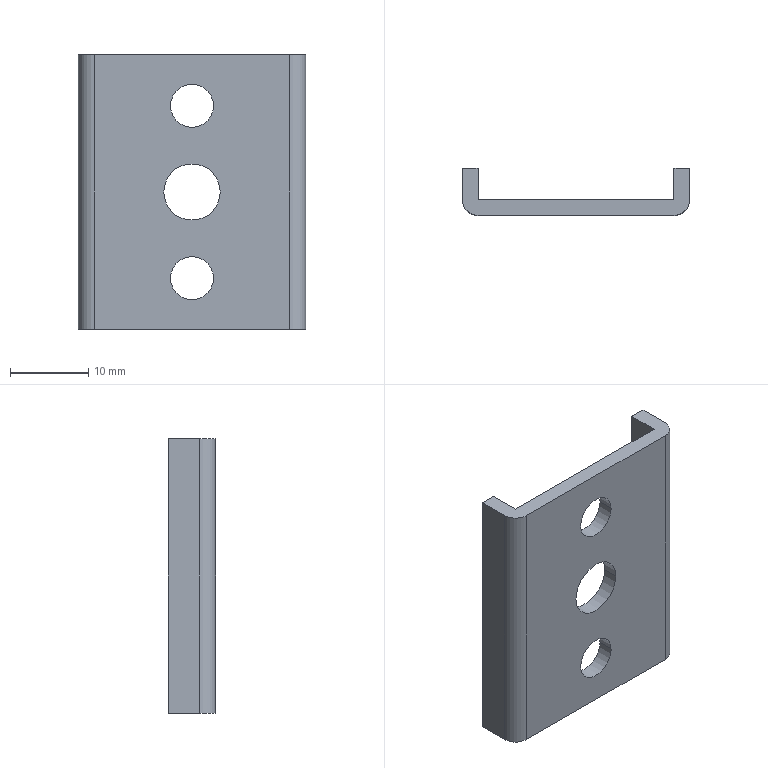Part | STEP file | _X2_751F4E45_X0_MS731-1_X2_8F_9 | 1 solid | 18 faces | box 29 x 6 x 35 mm | volume 2353 mm3 | plane 10 | cylinder 8 | commonest cylinder face diameters 5.5 x4 4 x2 7.2 x2
STEP:
#1=CARTESIAN_POINT('',(0.,0.,0.));
#2=DIRECTION('',(0.,0.,1.));
#3=DIRECTION('',(1.,0.,0.));
#4=AXIS2_PLACEMENT_3D('',#1,#2,#3);
#5=CARTESIAN_POINT('',(30.,20.681,-54.5));
#6=VERTEX_POINT('',#5);
#7=CARTESIAN_POINT('',(28.,20.681,-54.5));
#8=VERTEX_POINT('',#7);
#9=CARTESIAN_POINT('',(30.,20.681,-54.5));
#10=DIRECTION('',(-1.,0.,0.));
#11=VECTOR('',#10,1.);
#12=LINE('',#9,#11);
#13=CARTESIAN_POINT('',(15.5,20.681,-72.));
#14=DIRECTION('',(0.,-1.,0.));
#15=DIRECTION('',(1.,0.,0.));
#16=AXIS2_PLACEMENT_3D('',#13,#14,#15);
#17=PLANE('',#16);
#18=CARTESIAN_POINT('',(14.5,17.5));
#19=DIRECTION('',(-1.,0.));
#20=VECTOR('',#19,1.);
#21=LINE('',#18,#20);
#22=(GEOMETRIC_REPRESENTATION_CONTEXT(2)PARAMETRIC_REPRESENTATION_CONTEXT()REPRESENTATION_CONTEXT('',''));
#23=DEFINITIONAL_REPRESENTATION('',(#21),#22);
#24=PCURVE('',#17,#23);
#25=CARTESIAN_POINT('',(30.,20.681,-54.5));
#26=DIRECTION('',(0.,0.,1.));
#27=DIRECTION('',(1.,0.,0.));
#28=AXIS2_PLACEMENT_3D('',#25,#26,#27);
#29=PLANE('',#28);
#30=CARTESIAN_POINT('',(0.,0.));
#31=DIRECTION('',(-1.,0.));
#32=VECTOR('',#31,1.);
#33=LINE('',#30,#32);
#34=(GEOMETRIC_REPRESENTATION_CONTEXT(2)PARAMETRIC_REPRESENTATION_CONTEXT()REPRESENTATION_CONTEXT('',''));
#35=DEFINITIONAL_REPRESENTATION('',(#33),#34);
#36=PCURVE('',#29,#35);
#37=SURFACE_CURVE('',#12,(#24,#36),.PCURVE_S1.);
#38=EDGE_CURVE('',#6,#8,#37,.T.);
#39=ORIENTED_EDGE('',*,*,#38,.T.);
#40=CARTESIAN_POINT('',(28.,20.681,-89.5));
#41=VERTEX_POINT('',#40);
#42=CARTESIAN_POINT('',(28.,20.681,-54.5));
#43=DIRECTION('',(0.,0.,-1.));
#44=VECTOR('',#43,1.);
#45=LINE('',#42,#44);
#46=CARTESIAN_POINT('',(12.5,17.5));
#47=DIRECTION('',(0.,-1.));
#48=VECTOR('',#47,1.);
#49=LINE('',#46,#48);
#50=(GEOMETRIC_REPRESENTATION_CONTEXT(2)PARAMETRIC_REPRESENTATION_CONTEXT()REPRESENTATION_CONTEXT('',''));
#51=DEFINITIONAL_REPRESENTATION('',(#49),#50);
#52=PCURVE('',#17,#51);
#53=CARTESIAN_POINT('',(28.,16.681,-54.5));
#54=DIRECTION('',(1.,0.,0.));
#55=DIRECTION('',(0.,-1.,0.));
#56=AXIS2_PLACEMENT_3D('',#53,#54,#55);
#57=PLANE('',#56);
#58=CARTESIAN_POINT('',(-4.,0.));
#59=DIRECTION('',(0.,1.));
#60=VECTOR('',#59,1.);
#61=LINE('',#58,#60);
#62=(GEOMETRIC_REPRESENTATION_CONTEXT(2)PARAMETRIC_REPRESENTATION_CONTEXT()REPRESENTATION_CONTEXT('',''));
#63=DEFINITIONAL_REPRESENTATION('',(#61),#62);
#64=PCURVE('',#57,#63);
#65=SURFACE_CURVE('',#45,(#52,#64),.PCURVE_S1.);
#66=EDGE_CURVE('',#8,#41,#65,.T.);
#67=ORIENTED_EDGE('',*,*,#66,.T.);
#68=CARTESIAN_POINT('',(30.,20.681,-89.5));
#69=VERTEX_POINT('',#68);
#70=CARTESIAN_POINT('',(28.,20.681,-89.5));
#71=DIRECTION('',(1.,0.,0.));
#72=VECTOR('',#71,1.);
#73=LINE('',#70,#72);
#74=CARTESIAN_POINT('',(12.5,-17.5));
#75=DIRECTION('',(1.,0.));
#76=VECTOR('',#75,1.);
#77=LINE('',#74,#76);
#78=(GEOMETRIC_REPRESENTATION_CONTEXT(2)PARAMETRIC_REPRESENTATION_CONTEXT()REPRESENTATION_CONTEXT('',''));
#79=DEFINITIONAL_REPRESENTATION('',(#77),#78);
#80=PCURVE('',#17,#79);
#81=CARTESIAN_POINT('',(1.,20.681,-89.5));
#82=DIRECTION('',(0.,0.,-1.));
#83=DIRECTION('',(-1.,0.,0.));
#84=AXIS2_PLACEMENT_3D('',#81,#82,#83);
#85=PLANE('',#84);
#86=CARTESIAN_POINT('',(-27.,0.));
#87=DIRECTION('',(-1.,0.));
#88=VECTOR('',#87,1.);
#89=LINE('',#86,#88);
#90=(GEOMETRIC_REPRESENTATION_CONTEXT(2)PARAMETRIC_REPRESENTATION_CONTEXT()REPRESENTATION_CONTEXT('',''));
#91=DEFINITIONAL_REPRESENTATION('',(#89),#90);
#92=PCURVE('',#85,#91);
#93=SURFACE_CURVE('',#73,(#80,#92),.PCURVE_S1.);
#94=EDGE_CURVE('',#41,#69,#93,.T.);
#95=ORIENTED_EDGE('',*,*,#94,.T.);
#96=CARTESIAN_POINT('',(30.,20.681,-89.5));
#97=DIRECTION('',(0.,0.,1.));
#98=VECTOR('',#97,1.);
#99=LINE('',#96,#98);
#100=CARTESIAN_POINT('',(14.5,-17.5));
#101=DIRECTION('',(0.,1.));
#102=VECTOR('',#101,1.);
#103=LINE('',#100,#102);
#104=(GEOMETRIC_REPRESENTATION_CONTEXT(2)PARAMETRIC_REPRESENTATION_CONTEXT()REPRESENTATION_CONTEXT('',''));
#105=DEFINITIONAL_REPRESENTATION('',(#103),#104);
#106=PCURVE('',#17,#105);
#107=CARTESIAN_POINT('',(30.,20.681,-89.5));
#108=DIRECTION('',(1.,0.,0.));
#109=DIRECTION('',(0.,0.,-1.));
#110=AXIS2_PLACEMENT_3D('',#107,#108,#109);
#111=PLANE('',#110);
#112=CARTESIAN_POINT('',(0.,0.));
#113=DIRECTION('',(-1.,0.));
#114=VECTOR('',#113,1.);
#115=LINE('',#112,#114);
#116=(GEOMETRIC_REPRESENTATION_CONTEXT(2)PARAMETRIC_REPRESENTATION_CONTEXT()REPRESENTATION_CONTEXT('',''));
#117=DEFINITIONAL_REPRESENTATION('',(#115),#116);
#118=PCURVE('',#111,#117);
#119=SURFACE_CURVE('',#99,(#106,#118),.PCURVE_S1.);
#120=EDGE_CURVE('',#69,#6,#119,.T.);
#121=ORIENTED_EDGE('',*,*,#120,.T.);
#122=EDGE_LOOP('',(#39,#67,#95,#121));
#123=FACE_BOUND('',#122,.F.);
#124=ADVANCED_FACE('',(#123),#17,.F.);
#125=CARTESIAN_POINT('',(28.,14.681,-54.5));
#126=VERTEX_POINT('',#125);
#127=CARTESIAN_POINT('',(3.,14.681,-54.5));
#128=VERTEX_POINT('',#127);
#129=CARTESIAN_POINT('',(28.,14.681,-54.5));
#130=DIRECTION('',(-1.,0.,0.));
#131=VECTOR('',#130,1.);
#132=LINE('',#129,#131);
#133=CARTESIAN_POINT('',(-2.,-6.));
#134=DIRECTION('',(-1.,0.));
#135=VECTOR('',#134,1.);
#136=LINE('',#133,#135);
#137=(GEOMETRIC_REPRESENTATION_CONTEXT(2)PARAMETRIC_REPRESENTATION_CONTEXT()REPRESENTATION_CONTEXT('',''));
#138=DEFINITIONAL_REPRESENTATION('',(#136),#137);
#139=PCURVE('',#29,#138);
#140=CARTESIAN_POINT('',(15.5,14.681,-72.));
#141=DIRECTION('',(0.,-1.,0.));
#142=DIRECTION('',(1.,0.,0.));
#143=AXIS2_PLACEMENT_3D('',#140,#141,#142);
#144=PLANE('',#143);
#145=CARTESIAN_POINT('',(12.5,17.5));
#146=DIRECTION('',(-1.,0.));
#147=VECTOR('',#146,1.);
#148=LINE('',#145,#147);
#149=(GEOMETRIC_REPRESENTATION_CONTEXT(2)PARAMETRIC_REPRESENTATION_CONTEXT()REPRESENTATION_CONTEXT('',''));
#150=DEFINITIONAL_REPRESENTATION('',(#148),#149);
#151=PCURVE('',#144,#150);
#152=SURFACE_CURVE('',#132,(#139,#151),.PCURVE_S1.);
#153=EDGE_CURVE('',#126,#128,#152,.T.);
#154=ORIENTED_EDGE('',*,*,#153,.T.);
#155=CARTESIAN_POINT('',(1.,16.681,-54.5));
#156=VERTEX_POINT('',#155);
#157=CARTESIAN_POINT('',(3.,16.681,-54.5));
#158=DIRECTION('',(0.,0.,1.));
#159=DIRECTION('',(-1.,0.,0.));
#160=AXIS2_PLACEMENT_3D('',#157,#158,#159);
#161=CIRCLE('',#160,2.);
#162=CARTESIAN_POINT('',(-27.,-4.));
#163=DIRECTION('',(-1.,0.));
#164=AXIS2_PLACEMENT_2D('',#162,#163);
#165=CIRCLE('',#164,2.);
#166=(GEOMETRIC_REPRESENTATION_CONTEXT(2)PARAMETRIC_REPRESENTATION_CONTEXT()REPRESENTATION_CONTEXT('',''));
#167=DEFINITIONAL_REPRESENTATION('',(#165),#166);
#168=PCURVE('',#29,#167);
#169=CARTESIAN_POINT('',(3.,16.681,-54.425));
#170=DIRECTION('',(0.,0.,-1.));
#171=DIRECTION('',(0.,1.,0.));
#172=AXIS2_PLACEMENT_3D('',#169,#170,#171);
#173=CYLINDRICAL_SURFACE('',#172,2.);
#174=CARTESIAN_POINT('',(4.712,0.0754));
#175=DIRECTION('',(-1.,0.));
#176=VECTOR('',#175,1.);
#177=LINE('',#174,#176);
#178=(GEOMETRIC_REPRESENTATION_CONTEXT(2)PARAMETRIC_REPRESENTATION_CONTEXT()REPRESENTATION_CONTEXT('',''));
#179=DEFINITIONAL_REPRESENTATION('',(#177),#178);
#180=PCURVE('',#173,#179);
#181=SURFACE_CURVE('',#161,(#168,#180),.PCURVE_S1.);
#182=EDGE_CURVE('',#156,#128,#181,.T.);
#183=ORIENTED_EDGE('',*,*,#182,.F.);
#184=CARTESIAN_POINT('',(1.,20.681,-54.5));
#185=VERTEX_POINT('',#184);
#186=CARTESIAN_POINT('',(1.,20.681,-54.5));
#187=DIRECTION('',(0.,-1.,0.));
#188=VECTOR('',#187,1.);
#189=LINE('',#186,#188);
#190=CARTESIAN_POINT('',(-29.,0.));
#191=DIRECTION('',(0.,-1.));
#192=VECTOR('',#191,1.);
#193=LINE('',#190,#192);
#194=(GEOMETRIC_REPRESENTATION_CONTEXT(2)PARAMETRIC_REPRESENTATION_CONTEXT()REPRESENTATION_CONTEXT('',''));
#195=DEFINITIONAL_REPRESENTATION('',(#193),#194);
#196=PCURVE('',#29,#195);
#197=CARTESIAN_POINT('',(1.,20.681,-54.5));
#198=DIRECTION('',(-1.,0.,0.));
#199=DIRECTION('',(0.,0.,1.));
#200=AXIS2_PLACEMENT_3D('',#197,#198,#199);
#201=PLANE('',#200);
#202=CARTESIAN_POINT('',(0.,0.));
#203=DIRECTION('',(0.,-1.));
#204=VECTOR('',#203,1.);
#205=LINE('',#202,#204);
#206=(GEOMETRIC_REPRESENTATION_CONTEXT(2)PARAMETRIC_REPRESENTATION_CONTEXT()REPRESENTATION_CONTEXT('',''));
#207=DEFINITIONAL_REPRESENTATION('',(#205),#206);
#208=PCURVE('',#201,#207);
#209=SURFACE_CURVE('',#189,(#196,#208),.PCURVE_S1.);
#210=EDGE_CURVE('',#185,#156,#209,.T.);
#211=ORIENTED_EDGE('',*,*,#210,.F.);
#212=CARTESIAN_POINT('',(3.,20.681,-54.5));
#213=VERTEX_POINT('',#212);
#214=CARTESIAN_POINT('',(3.,20.681,-54.5));
#215=DIRECTION('',(-1.,0.,0.));
#216=VECTOR('',#215,1.);
#217=LINE('',#214,#216);
#218=CARTESIAN_POINT('',(-27.,0.));
#219=DIRECTION('',(-1.,0.));
#220=VECTOR('',#219,1.);
#221=LINE('',#218,#220);
#222=(GEOMETRIC_REPRESENTATION_CONTEXT(2)PARAMETRIC_REPRESENTATION_CONTEXT()REPRESENTATION_CONTEXT('',''));
#223=DEFINITIONAL_REPRESENTATION('',(#221),#222);
#224=PCURVE('',#29,#223);
#225=CARTESIAN_POINT('',(15.5,20.681,-72.));
#226=DIRECTION('',(0.,-1.,0.));
#227=DIRECTION('',(1.,0.,0.));
#228=AXIS2_PLACEMENT_3D('',#225,#226,#227);
#229=PLANE('',#228);
#230=CARTESIAN_POINT('',(-12.5,17.5));
#231=DIRECTION('',(-1.,0.));
#232=VECTOR('',#231,1.);
#233=LINE('',#230,#232);
#234=(GEOMETRIC_REPRESENTATION_CONTEXT(2)PARAMETRIC_REPRESENTATION_CONTEXT()REPRESENTATION_CONTEXT('',''));
#235=DEFINITIONAL_REPRESENTATION('',(#233),#234);
#236=PCURVE('',#229,#235);
#237=SURFACE_CURVE('',#217,(#224,#236),.PCURVE_S1.);
#238=EDGE_CURVE('',#213,#185,#237,.T.);
#239=ORIENTED_EDGE('',*,*,#238,.F.);
#240=CARTESIAN_POINT('',(3.,16.681,-54.5));
#241=VERTEX_POINT('',#240);
#242=CARTESIAN_POINT('',(3.,20.681,-54.5));
#243=DIRECTION('',(0.,-1.,0.));
#244=VECTOR('',#243,1.);
#245=LINE('',#242,#244);
#246=CARTESIAN_POINT('',(-27.,0.));
#247=DIRECTION('',(0.,-1.));
#248=VECTOR('',#247,1.);
#249=LINE('',#246,#248);
#250=(GEOMETRIC_REPRESENTATION_CONTEXT(2)PARAMETRIC_REPRESENTATION_CONTEXT()REPRESENTATION_CONTEXT('',''));
#251=DEFINITIONAL_REPRESENTATION('',(#249),#250);
#252=PCURVE('',#29,#251);
#253=CARTESIAN_POINT('',(3.,20.681,-54.5));
#254=DIRECTION('',(-1.,0.,0.));
#255=DIRECTION('',(0.,1.,0.));
#256=AXIS2_PLACEMENT_3D('',#253,#254,#255);
#257=PLANE('',#256);
#258=CARTESIAN_POINT('',(0.,0.));
#259=DIRECTION('',(-1.,0.));
#260=VECTOR('',#259,1.);
#261=LINE('',#258,#260);
#262=(GEOMETRIC_REPRESENTATION_CONTEXT(2)PARAMETRIC_REPRESENTATION_CONTEXT()REPRESENTATION_CONTEXT('',''));
#263=DEFINITIONAL_REPRESENTATION('',(#261),#262);
#264=PCURVE('',#257,#263);
#265=SURFACE_CURVE('',#245,(#252,#264),.PCURVE_S1.);
#266=EDGE_CURVE('',#213,#241,#265,.T.);
#267=ORIENTED_EDGE('',*,*,#266,.T.);
#268=CARTESIAN_POINT('',(28.,16.681,-54.5));
#269=VERTEX_POINT('',#268);
#270=CARTESIAN_POINT('',(3.,16.681,-54.5));
#271=DIRECTION('',(1.,0.,0.));
#272=VECTOR('',#271,1.);
#273=LINE('',#270,#272);
#274=CARTESIAN_POINT('',(-27.,-4.));
#275=DIRECTION('',(1.,0.));
#276=VECTOR('',#275,1.);
#277=LINE('',#274,#276);
#278=(GEOMETRIC_REPRESENTATION_CONTEXT(2)PARAMETRIC_REPRESENTATION_CONTEXT()REPRESENTATION_CONTEXT('',''));
#279=DEFINITIONAL_REPRESENTATION('',(#277),#278);
#280=PCURVE('',#29,#279);
#281=CARTESIAN_POINT('',(3.,16.681,-54.5));
#282=DIRECTION('',(0.,-1.,0.));
#283=DIRECTION('',(-1.,0.,0.));
#284=AXIS2_PLACEMENT_3D('',#281,#282,#283);
#285=PLANE('',#284);
#286=CARTESIAN_POINT('',(0.,0.));
#287=DIRECTION('',(-1.,0.));
#288=VECTOR('',#287,1.);
#289=LINE('',#286,#288);
#290=(GEOMETRIC_REPRESENTATION_CONTEXT(2)PARAMETRIC_REPRESENTATION_CONTEXT()REPRESENTATION_CONTEXT('',''));
#291=DEFINITIONAL_REPRESENTATION('',(#289),#290);
#292=PCURVE('',#285,#291);
#293=SURFACE_CURVE('',#273,(#280,#292),.PCURVE_S1.);
#294=EDGE_CURVE('',#241,#269,#293,.T.);
#295=ORIENTED_EDGE('',*,*,#294,.T.);
#296=CARTESIAN_POINT('',(28.,20.681,-54.5));
#297=DIRECTION('',(0.,-1.,0.));
#298=VECTOR('',#297,1.);
#299=LINE('',#296,#298);
#300=CARTESIAN_POINT('',(-2.,0.));
#301=DIRECTION('',(0.,-1.));
#302=VECTOR('',#301,1.);
#303=LINE('',#300,#302);
#304=(GEOMETRIC_REPRESENTATION_CONTEXT(2)PARAMETRIC_REPRESENTATION_CONTEXT()REPRESENTATION_CONTEXT('',''));
#305=DEFINITIONAL_REPRESENTATION('',(#303),#304);
#306=PCURVE('',#29,#305);
#307=CARTESIAN_POINT('',(-4.,0.));
#308=DIRECTION('',(1.,0.));
#309=VECTOR('',#308,1.);
#310=LINE('',#307,#309);
#311=(GEOMETRIC_REPRESENTATION_CONTEXT(2)PARAMETRIC_REPRESENTATION_CONTEXT()REPRESENTATION_CONTEXT('',''));
#312=DEFINITIONAL_REPRESENTATION('',(#310),#311);
#313=PCURVE('',#57,#312);
#314=SURFACE_CURVE('',#299,(#306,#313),.PCURVE_S1.);
#315=EDGE_CURVE('',#8,#269,#314,.T.);
#316=ORIENTED_EDGE('',*,*,#315,.F.);
#317=ORIENTED_EDGE('',*,*,#38,.F.);
#318=CARTESIAN_POINT('',(30.,16.681,-54.5));
#319=VERTEX_POINT('',#318);
#320=CARTESIAN_POINT('',(30.,20.681,-54.5));
#321=DIRECTION('',(0.,-1.,0.));
#322=VECTOR('',#321,1.);
#323=LINE('',#320,#322);
#324=CARTESIAN_POINT('',(0.,0.));
#325=DIRECTION('',(0.,-1.));
#326=VECTOR('',#325,1.);
#327=LINE('',#324,#326);
#328=(GEOMETRIC_REPRESENTATION_CONTEXT(2)PARAMETRIC_REPRESENTATION_CONTEXT()REPRESENTATION_CONTEXT('',''));
#329=DEFINITIONAL_REPRESENTATION('',(#327),#328);
#330=PCURVE('',#29,#329);
#331=CARTESIAN_POINT('',(-35.,0.));
#332=DIRECTION('',(0.,-1.));
#333=VECTOR('',#332,1.);
#334=LINE('',#331,#333);
#335=(GEOMETRIC_REPRESENTATION_CONTEXT(2)PARAMETRIC_REPRESENTATION_CONTEXT()REPRESENTATION_CONTEXT('',''));
#336=DEFINITIONAL_REPRESENTATION('',(#334),#335);
#337=PCURVE('',#111,#336);
#338=SURFACE_CURVE('',#323,(#330,#337),.PCURVE_S1.);
#339=EDGE_CURVE('',#6,#319,#338,.T.);
#340=ORIENTED_EDGE('',*,*,#339,.T.);
#341=CARTESIAN_POINT('',(28.,16.681,-54.5));
#342=DIRECTION('',(0.,0.,1.));
#343=DIRECTION('',(0.,-1.,0.));
#344=AXIS2_PLACEMENT_3D('',#341,#342,#343);
#345=CIRCLE('',#344,2.);
#346=CARTESIAN_POINT('',(-2.,-4.));
#347=DIRECTION('',(0.,-1.));
#348=AXIS2_PLACEMENT_2D('',#346,#347);
#349=CIRCLE('',#348,2.);
#350=(GEOMETRIC_REPRESENTATION_CONTEXT(2)PARAMETRIC_REPRESENTATION_CONTEXT()REPRESENTATION_CONTEXT('',''));
#351=DEFINITIONAL_REPRESENTATION('',(#349),#350);
#352=PCURVE('',#29,#351);
#353=CARTESIAN_POINT('',(28.,16.681,-89.577));
#354=DIRECTION('',(0.,0.,1.));
#355=DIRECTION('',(0.,1.,0.));
#356=AXIS2_PLACEMENT_3D('',#353,#354,#355);
#357=CYLINDRICAL_SURFACE('',#356,2.);
#358=CARTESIAN_POINT('',(3.142,35.077));
#359=DIRECTION('',(1.,0.));
#360=VECTOR('',#359,1.);
#361=LINE('',#358,#360);
#362=(GEOMETRIC_REPRESENTATION_CONTEXT(2)PARAMETRIC_REPRESENTATION_CONTEXT()REPRESENTATION_CONTEXT('',''));
#363=DEFINITIONAL_REPRESENTATION('',(#361),#362);
#364=PCURVE('',#357,#363);
#365=SURFACE_CURVE('',#345,(#352,#364),.PCURVE_S1.);
#366=EDGE_CURVE('',#126,#319,#365,.T.);
#367=ORIENTED_EDGE('',*,*,#366,.F.);
#368=EDGE_LOOP('',(#154,#183,#211,#239,#267,#295,#316,#317,#340,#367));
#369=FACE_BOUND('',#368,.F.);
#370=ADVANCED_FACE('',(#369),#29,.T.);
#371=CARTESIAN_POINT('',(3.,14.681,-89.5));
#372=VERTEX_POINT('',#371);
#373=CARTESIAN_POINT('',(28.,14.681,-89.5));
#374=VERTEX_POINT('',#373);
#375=CARTESIAN_POINT('',(3.,14.681,-89.5));
#376=DIRECTION('',(1.,0.,0.));
#377=VECTOR('',#376,1.);
#378=LINE('',#375,#377);
#379=CARTESIAN_POINT('',(-12.5,-17.5));
#380=DIRECTION('',(1.,0.));
#381=VECTOR('',#380,1.);
#382=LINE('',#379,#381);
#383=(GEOMETRIC_REPRESENTATION_CONTEXT(2)PARAMETRIC_REPRESENTATION_CONTEXT()REPRESENTATION_CONTEXT('',''));
#384=DEFINITIONAL_REPRESENTATION('',(#382),#383);
#385=PCURVE('',#144,#384);
#386=CARTESIAN_POINT('',(-2.,-6.));
#387=DIRECTION('',(-1.,0.));
#388=VECTOR('',#387,1.);
#389=LINE('',#386,#388);
#390=(GEOMETRIC_REPRESENTATION_CONTEXT(2)PARAMETRIC_REPRESENTATION_CONTEXT()REPRESENTATION_CONTEXT('',''));
#391=DEFINITIONAL_REPRESENTATION('',(#389),#390);
#392=PCURVE('',#85,#391);
#393=SURFACE_CURVE('',#378,(#385,#392),.PCURVE_S1.);
#394=EDGE_CURVE('',#372,#374,#393,.T.);
#395=ORIENTED_EDGE('',*,*,#394,.F.);
#396=CARTESIAN_POINT('',(3.,14.681,-89.5));
#397=DIRECTION('',(0.,0.,1.));
#398=VECTOR('',#397,1.);
#399=LINE('',#396,#398);
#400=CARTESIAN_POINT('',(-12.5,-17.5));
#401=DIRECTION('',(0.,1.));
#402=VECTOR('',#401,1.);
#403=LINE('',#400,#402);
#404=(GEOMETRIC_REPRESENTATION_CONTEXT(2)PARAMETRIC_REPRESENTATION_CONTEXT()REPRESENTATION_CONTEXT('',''));
#405=DEFINITIONAL_REPRESENTATION('',(#403),#404);
#406=PCURVE('',#144,#405);
#407=CARTESIAN_POINT('',(3.142,35.075));
#408=DIRECTION('',(0.,-1.));
#409=VECTOR('',#408,1.);
#410=LINE('',#407,#409);
#411=(GEOMETRIC_REPRESENTATION_CONTEXT(2)PARAMETRIC_REPRESENTATION_CONTEXT()REPRESENTATION_CONTEXT('',''));
#412=DEFINITIONAL_REPRESENTATION('',(#410),#411);
#413=PCURVE('',#173,#412);
#414=SURFACE_CURVE('',#399,(#406,#413),.PCURVE_S1.);
#415=EDGE_CURVE('',#372,#128,#414,.T.);
#416=ORIENTED_EDGE('',*,*,#415,.T.);
#417=ORIENTED_EDGE('',*,*,#153,.F.);
#418=CARTESIAN_POINT('',(28.,14.681,-54.5));
#419=DIRECTION('',(0.,0.,-1.));
#420=VECTOR('',#419,1.);
#421=LINE('',#418,#420);
#422=CARTESIAN_POINT('',(12.5,17.5));
#423=DIRECTION('',(0.,-1.));
#424=VECTOR('',#423,1.);
#425=LINE('',#422,#424);
#426=(GEOMETRIC_REPRESENTATION_CONTEXT(2)PARAMETRIC_REPRESENTATION_CONTEXT()REPRESENTATION_CONTEXT('',''));
#427=DEFINITIONAL_REPRESENTATION('',(#425),#426);
#428=PCURVE('',#144,#427);
#429=CARTESIAN_POINT('',(3.142,35.077));
#430=DIRECTION('',(0.,-1.));
#431=VECTOR('',#430,1.);
#432=LINE('',#429,#431);
#433=(GEOMETRIC_REPRESENTATION_CONTEXT(2)PARAMETRIC_REPRESENTATION_CONTEXT()REPRESENTATION_CONTEXT('',''));
#434=DEFINITIONAL_REPRESENTATION('',(#432),#433);
#435=PCURVE('',#357,#434);
#436=SURFACE_CURVE('',#421,(#428,#435),.PCURVE_S1.);
#437=EDGE_CURVE('',#126,#374,#436,.T.);
#438=ORIENTED_EDGE('',*,*,#437,.T.);
#439=EDGE_LOOP('',(#395,#416,#417,#438));
#440=FACE_BOUND('',#439,.F.);
#441=CARTESIAN_POINT('',(18.25,14.681,-83.));
#442=VERTEX_POINT('',#441);
#443=CARTESIAN_POINT('',(12.75,14.681,-83.));
#444=VERTEX_POINT('',#443);
#445=CARTESIAN_POINT('',(15.5,14.681,-83.));
#446=DIRECTION('',(0.,1.,0.));
#447=DIRECTION('',(1.,0.,0.));
#448=AXIS2_PLACEMENT_3D('',#445,#446,#447);
#449=CIRCLE('',#448,2.75);
#450=CARTESIAN_POINT('',(2.75,-11.));
#451=CARTESIAN_POINT('',(2.75,-15.763));
#452=CARTESIAN_POINT('',(-1.375,-13.382));
#453=CARTESIAN_POINT('',(-5.5,-11.));
#454=CARTESIAN_POINT('',(-1.375,-8.618));
#455=CARTESIAN_POINT('',(2.75,-6.237));
#456=CARTESIAN_POINT('',(2.75,-11.));
#457=(BOUNDED_CURVE()B_SPLINE_CURVE(2,(#450,#451,#452,#453,#454,#455,#456),.UNSPECIFIED.,.T.,.F.)B_SPLINE_CURVE_WITH_KNOTS((1,2,2,2,2,1),(-2.094,0.,2.094,4.189,6.283,8.378),.UNSPECIFIED.)CURVE()GEOMETRIC_REPRESENTATION_ITEM()RATIONAL_B_SPLINE_CURVE((1.,0.5,1.,0.5,1.,0.5,1.))REPRESENTATION_ITEM(''));
#458=(GEOMETRIC_REPRESENTATION_CONTEXT(2)PARAMETRIC_REPRESENTATION_CONTEXT()REPRESENTATION_CONTEXT('',''));
#459=DEFINITIONAL_REPRESENTATION('',(#457),#458);
#460=PCURVE('',#144,#459);
#461=CARTESIAN_POINT('',(15.5,20.681,-83.));
#462=DIRECTION('',(0.,-1.,0.));
#463=DIRECTION('',(1.,0.,0.));
#464=AXIS2_PLACEMENT_3D('',#461,#462,#463);
#465=CYLINDRICAL_SURFACE('',#464,2.75);
#466=CARTESIAN_POINT('',(6.283,6.));
#467=DIRECTION('',(-1.,0.));
#468=VECTOR('',#467,1.);
#469=LINE('',#466,#468);
#470=(GEOMETRIC_REPRESENTATION_CONTEXT(2)PARAMETRIC_REPRESENTATION_CONTEXT()REPRESENTATION_CONTEXT('',''));
#471=DEFINITIONAL_REPRESENTATION('',(#469),#470);
#472=PCURVE('',#465,#471);
#473=SURFACE_CURVE('',#449,(#460,#472),.PCURVE_S1.);
#474=EDGE_CURVE('',#442,#444,#473,.T.);
#475=ORIENTED_EDGE('',*,*,#474,.F.);
#476=CARTESIAN_POINT('',(15.5,14.681,-83.));
#477=DIRECTION('',(0.,1.,0.));
#478=DIRECTION('',(-1.,0.,0.));
#479=AXIS2_PLACEMENT_3D('',#476,#477,#478);
#480=CIRCLE('',#479,2.75);
#481=CARTESIAN_POINT('',(-2.75,-11.));
#482=CARTESIAN_POINT('',(-2.75,-6.237));
#483=CARTESIAN_POINT('',(1.375,-8.618));
#484=CARTESIAN_POINT('',(5.5,-11.));
#485=CARTESIAN_POINT('',(1.375,-13.382));
#486=CARTESIAN_POINT('',(-2.75,-15.763));
#487=CARTESIAN_POINT('',(-2.75,-11.));
#488=(BOUNDED_CURVE()B_SPLINE_CURVE(2,(#481,#482,#483,#484,#485,#486,#487),.UNSPECIFIED.,.T.,.F.)B_SPLINE_CURVE_WITH_KNOTS((1,2,2,2,2,1),(-2.094,0.,2.094,4.189,6.283,8.378),.UNSPECIFIED.)CURVE()GEOMETRIC_REPRESENTATION_ITEM()RATIONAL_B_SPLINE_CURVE((1.,0.5,1.,0.5,1.,0.5,1.))REPRESENTATION_ITEM(''));
#489=(GEOMETRIC_REPRESENTATION_CONTEXT(2)PARAMETRIC_REPRESENTATION_CONTEXT()REPRESENTATION_CONTEXT('',''));
#490=DEFINITIONAL_REPRESENTATION('',(#488),#489);
#491=PCURVE('',#144,#490);
#492=CARTESIAN_POINT('',(15.5,20.681,-83.));
#493=DIRECTION('',(0.,-1.,0.));
#494=DIRECTION('',(1.,0.,0.));
#495=AXIS2_PLACEMENT_3D('',#492,#493,#494);
#496=CYLINDRICAL_SURFACE('',#495,2.75);
#497=CARTESIAN_POINT('',(3.142,6.));
#498=DIRECTION('',(-1.,0.));
#499=VECTOR('',#498,1.);
#500=LINE('',#497,#499);
#501=(GEOMETRIC_REPRESENTATION_CONTEXT(2)PARAMETRIC_REPRESENTATION_CONTEXT()REPRESENTATION_CONTEXT('',''));
#502=DEFINITIONAL_REPRESENTATION('',(#500),#501);
#503=PCURVE('',#496,#502);
#504=SURFACE_CURVE('',#480,(#491,#503),.PCURVE_S1.);
#505=EDGE_CURVE('',#444,#442,#504,.T.);
#506=ORIENTED_EDGE('',*,*,#505,.F.);
#507=EDGE_LOOP('',(#475,#506));
#508=FACE_BOUND('',#507,.F.);
#509=CARTESIAN_POINT('',(18.25,14.681,-61.));
#510=VERTEX_POINT('',#509);
#511=CARTESIAN_POINT('',(12.75,14.681,-61.));
#512=VERTEX_POINT('',#511);
#513=CARTESIAN_POINT('',(15.5,14.681,-61.));
#514=DIRECTION('',(0.,1.,0.));
#515=DIRECTION('',(1.,0.,0.));
#516=AXIS2_PLACEMENT_3D('',#513,#514,#515);
#517=CIRCLE('',#516,2.75);
#518=CARTESIAN_POINT('',(2.75,11.));
#519=CARTESIAN_POINT('',(2.75,6.237));
#520=CARTESIAN_POINT('',(-1.375,8.618));
#521=CARTESIAN_POINT('',(-5.5,11.));
#522=CARTESIAN_POINT('',(-1.375,13.382));
#523=CARTESIAN_POINT('',(2.75,15.763));
#524=CARTESIAN_POINT('',(2.75,11.));
#525=(BOUNDED_CURVE()B_SPLINE_CURVE(2,(#518,#519,#520,#521,#522,#523,#524),.UNSPECIFIED.,.T.,.F.)B_SPLINE_CURVE_WITH_KNOTS((1,2,2,2,2,1),(-2.094,0.,2.094,4.189,6.283,8.378),.UNSPECIFIED.)CURVE()GEOMETRIC_REPRESENTATION_ITEM()RATIONAL_B_SPLINE_CURVE((1.,0.5,1.,0.5,1.,0.5,1.))REPRESENTATION_ITEM(''));
#526=(GEOMETRIC_REPRESENTATION_CONTEXT(2)PARAMETRIC_REPRESENTATION_CONTEXT()REPRESENTATION_CONTEXT('',''));
#527=DEFINITIONAL_REPRESENTATION('',(#525),#526);
#528=PCURVE('',#144,#527);
#529=CARTESIAN_POINT('',(15.5,20.681,-61.));
#530=DIRECTION('',(0.,-1.,0.));
#531=DIRECTION('',(1.,0.,0.));
#532=AXIS2_PLACEMENT_3D('',#529,#530,#531);
#533=CYLINDRICAL_SURFACE('',#532,2.75);
#534=CARTESIAN_POINT('',(6.283,6.));
#535=DIRECTION('',(-1.,0.));
#536=VECTOR('',#535,1.);
#537=LINE('',#534,#536);
#538=(GEOMETRIC_REPRESENTATION_CONTEXT(2)PARAMETRIC_REPRESENTATION_CONTEXT()REPRESENTATION_CONTEXT('',''));
#539=DEFINITIONAL_REPRESENTATION('',(#537),#538);
#540=PCURVE('',#533,#539);
#541=SURFACE_CURVE('',#517,(#528,#540),.PCURVE_S1.);
#542=EDGE_CURVE('',#510,#512,#541,.T.);
#543=ORIENTED_EDGE('',*,*,#542,.F.);
#544=CARTESIAN_POINT('',(15.5,14.681,-61.));
#545=DIRECTION('',(0.,1.,0.));
#546=DIRECTION('',(-1.,0.,0.));
#547=AXIS2_PLACEMENT_3D('',#544,#545,#546);
#548=CIRCLE('',#547,2.75);
#549=CARTESIAN_POINT('',(-2.75,11.));
#550=CARTESIAN_POINT('',(-2.75,15.763));
#551=CARTESIAN_POINT('',(1.375,13.382));
#552=CARTESIAN_POINT('',(5.5,11.));
#553=CARTESIAN_POINT('',(1.375,8.618));
#554=CARTESIAN_POINT('',(-2.75,6.237));
#555=CARTESIAN_POINT('',(-2.75,11.));
#556=(BOUNDED_CURVE()B_SPLINE_CURVE(2,(#549,#550,#551,#552,#553,#554,#555),.UNSPECIFIED.,.T.,.F.)B_SPLINE_CURVE_WITH_KNOTS((1,2,2,2,2,1),(-2.094,0.,2.094,4.189,6.283,8.378),.UNSPECIFIED.)CURVE()GEOMETRIC_REPRESENTATION_ITEM()RATIONAL_B_SPLINE_CURVE((1.,0.5,1.,0.5,1.,0.5,1.))REPRESENTATION_ITEM(''));
#557=(GEOMETRIC_REPRESENTATION_CONTEXT(2)PARAMETRIC_REPRESENTATION_CONTEXT()REPRESENTATION_CONTEXT('',''));
#558=DEFINITIONAL_REPRESENTATION('',(#556),#557);
#559=PCURVE('',#144,#558);
#560=CARTESIAN_POINT('',(15.5,20.681,-61.));
#561=DIRECTION('',(0.,-1.,0.));
#562=DIRECTION('',(1.,0.,0.));
#563=AXIS2_PLACEMENT_3D('',#560,#561,#562);
#564=CYLINDRICAL_SURFACE('',#563,2.75);
#565=CARTESIAN_POINT('',(3.142,6.));
#566=DIRECTION('',(-1.,0.));
#567=VECTOR('',#566,1.);
#568=LINE('',#565,#567);
#569=(GEOMETRIC_REPRESENTATION_CONTEXT(2)PARAMETRIC_REPRESENTATION_CONTEXT()REPRESENTATION_CONTEXT('',''));
#570=DEFINITIONAL_REPRESENTATION('',(#568),#569);
#571=PCURVE('',#564,#570);
#572=SURFACE_CURVE('',#548,(#559,#571),.PCURVE_S1.);
#573=EDGE_CURVE('',#512,#510,#572,.T.);
#574=ORIENTED_EDGE('',*,*,#573,.F.);
#575=EDGE_LOOP('',(#543,#574));
#576=FACE_BOUND('',#575,.F.);
#577=CARTESIAN_POINT('',(19.1,14.681,-72.));
#578=VERTEX_POINT('',#577);
#579=CARTESIAN_POINT('',(11.9,14.681,-72.));
#580=VERTEX_POINT('',#579);
#581=CARTESIAN_POINT('',(15.5,14.681,-72.));
#582=DIRECTION('',(0.,1.,0.));
#583=DIRECTION('',(1.,0.,0.));
#584=AXIS2_PLACEMENT_3D('',#581,#582,#583);
#585=CIRCLE('',#584,3.6);
#586=CARTESIAN_POINT('',(3.6,0.));
#587=CARTESIAN_POINT('',(3.6,-6.235));
#588=CARTESIAN_POINT('',(-1.8,-3.118));
#589=CARTESIAN_POINT('',(-7.2,0.));
#590=CARTESIAN_POINT('',(-1.8,3.118));
#591=CARTESIAN_POINT('',(3.6,6.235));
#592=CARTESIAN_POINT('',(3.6,0.));
#593=(BOUNDED_CURVE()B_SPLINE_CURVE(2,(#586,#587,#588,#589,#590,#591,#592),.UNSPECIFIED.,.T.,.F.)B_SPLINE_CURVE_WITH_KNOTS((1,2,2,2,2,1),(-2.094,0.,2.094,4.189,6.283,8.378),.UNSPECIFIED.)CURVE()GEOMETRIC_REPRESENTATION_ITEM()RATIONAL_B_SPLINE_CURVE((1.,0.5,1.,0.5,1.,0.5,1.))REPRESENTATION_ITEM(''));
#594=(GEOMETRIC_REPRESENTATION_CONTEXT(2)PARAMETRIC_REPRESENTATION_CONTEXT()REPRESENTATION_CONTEXT('',''));
#595=DEFINITIONAL_REPRESENTATION('',(#593),#594);
#596=PCURVE('',#144,#595);
#597=CARTESIAN_POINT('',(15.5,20.681,-72.));
#598=DIRECTION('',(0.,-1.,0.));
#599=DIRECTION('',(1.,0.,0.));
#600=AXIS2_PLACEMENT_3D('',#597,#598,#599);
#601=CYLINDRICAL_SURFACE('',#600,3.6);
#602=CARTESIAN_POINT('',(6.283,6.));
#603=DIRECTION('',(-1.,0.));
#604=VECTOR('',#603,1.);
#605=LINE('',#602,#604);
#606=(GEOMETRIC_REPRESENTATION_CONTEXT(2)PARAMETRIC_REPRESENTATION_CONTEXT()REPRESENTATION_CONTEXT('',''));
#607=DEFINITIONAL_REPRESENTATION('',(#605),#606);
#608=PCURVE('',#601,#607);
#609=SURFACE_CURVE('',#585,(#596,#608),.PCURVE_S1.);
#610=EDGE_CURVE('',#578,#580,#609,.T.);
#611=ORIENTED_EDGE('',*,*,#610,.F.);
#612=CARTESIAN_POINT('',(15.5,14.681,-72.));
#613=DIRECTION('',(0.,1.,0.));
#614=DIRECTION('',(-1.,0.,0.));
#615=AXIS2_PLACEMENT_3D('',#612,#613,#614);
#616=CIRCLE('',#615,3.6);
#617=CARTESIAN_POINT('',(-3.6,0.));
#618=CARTESIAN_POINT('',(-3.6,6.235));
#619=CARTESIAN_POINT('',(1.8,3.118));
#620=CARTESIAN_POINT('',(7.2,0.));
#621=CARTESIAN_POINT('',(1.8,-3.118));
#622=CARTESIAN_POINT('',(-3.6,-6.235));
#623=CARTESIAN_POINT('',(-3.6,0.));
#624=(BOUNDED_CURVE()B_SPLINE_CURVE(2,(#617,#618,#619,#620,#621,#622,#623),.UNSPECIFIED.,.T.,.F.)B_SPLINE_CURVE_WITH_KNOTS((1,2,2,2,2,1),(-2.094,0.,2.094,4.189,6.283,8.378),.UNSPECIFIED.)CURVE()GEOMETRIC_REPRESENTATION_ITEM()RATIONAL_B_SPLINE_CURVE((1.,0.5,1.,0.5,1.,0.5,1.))REPRESENTATION_ITEM(''));
#625=(GEOMETRIC_REPRESENTATION_CONTEXT(2)PARAMETRIC_REPRESENTATION_CONTEXT()REPRESENTATION_CONTEXT('',''));
#626=DEFINITIONAL_REPRESENTATION('',(#624),#625);
#627=PCURVE('',#144,#626);
#628=CARTESIAN_POINT('',(15.5,20.681,-72.));
#629=DIRECTION('',(0.,-1.,0.));
#630=DIRECTION('',(1.,0.,0.));
#631=AXIS2_PLACEMENT_3D('',#628,#629,#630);
#632=CYLINDRICAL_SURFACE('',#631,3.6);
#633=CARTESIAN_POINT('',(3.142,6.));
#634=DIRECTION('',(-1.,0.));
#635=VECTOR('',#634,1.);
#636=LINE('',#633,#635);
#637=(GEOMETRIC_REPRESENTATION_CONTEXT(2)PARAMETRIC_REPRESENTATION_CONTEXT()REPRESENTATION_CONTEXT('',''));
#638=DEFINITIONAL_REPRESENTATION('',(#636),#637);
#639=PCURVE('',#632,#638);
#640=SURFACE_CURVE('',#616,(#627,#639),.PCURVE_S1.);
#641=EDGE_CURVE('',#580,#578,#640,.T.);
#642=ORIENTED_EDGE('',*,*,#641,.F.);
#643=EDGE_LOOP('',(#611,#642));
#644=FACE_BOUND('',#643,.F.);
#645=ADVANCED_FACE('',(#440,#508,#576,#644),#144,.T.);
#646=CARTESIAN_POINT('',(1.,20.681,-89.5));
#647=VERTEX_POINT('',#646);
#648=CARTESIAN_POINT('',(1.,16.681,-89.5));
#649=VERTEX_POINT('',#648);
#650=CARTESIAN_POINT('',(1.,20.681,-89.5));
#651=DIRECTION('',(0.,-1.,0.));
#652=VECTOR('',#651,1.);
#653=LINE('',#650,#652);
#654=CARTESIAN_POINT('',(0.,0.));
#655=DIRECTION('',(0.,-1.));
#656=VECTOR('',#655,1.);
#657=LINE('',#654,#656);
#658=(GEOMETRIC_REPRESENTATION_CONTEXT(2)PARAMETRIC_REPRESENTATION_CONTEXT()REPRESENTATION_CONTEXT('',''));
#659=DEFINITIONAL_REPRESENTATION('',(#657),#658);
#660=PCURVE('',#85,#659);
#661=CARTESIAN_POINT('',(-35.,0.));
#662=DIRECTION('',(0.,-1.));
#663=VECTOR('',#662,1.);
#664=LINE('',#661,#663);
#665=(GEOMETRIC_REPRESENTATION_CONTEXT(2)PARAMETRIC_REPRESENTATION_CONTEXT()REPRESENTATION_CONTEXT('',''));
#666=DEFINITIONAL_REPRESENTATION('',(#664),#665);
#667=PCURVE('',#201,#666);
#668=SURFACE_CURVE('',#653,(#660,#667),.PCURVE_S1.);
#669=EDGE_CURVE('',#647,#649,#668,.T.);
#670=ORIENTED_EDGE('',*,*,#669,.T.);
#671=CARTESIAN_POINT('',(3.,16.681,-89.5));
#672=DIRECTION('',(0.,0.,-1.));
#673=DIRECTION('',(0.,-1.,0.));
#674=AXIS2_PLACEMENT_3D('',#671,#672,#673);
#675=CIRCLE('',#674,2.);
#676=CARTESIAN_POINT('',(-2.,-4.));
#677=DIRECTION('',(0.,-1.));
#678=AXIS2_PLACEMENT_2D('',#676,#677);
#679=CIRCLE('',#678,2.);
#680=(GEOMETRIC_REPRESENTATION_CONTEXT(2)PARAMETRIC_REPRESENTATION_CONTEXT()REPRESENTATION_CONTEXT('',''));
#681=DEFINITIONAL_REPRESENTATION('',(#679),#680);
#682=PCURVE('',#85,#681);
#683=CARTESIAN_POINT('',(3.142,35.075));
#684=DIRECTION('',(1.,0.));
#685=VECTOR('',#684,1.);
#686=LINE('',#683,#685);
#687=(GEOMETRIC_REPRESENTATION_CONTEXT(2)PARAMETRIC_REPRESENTATION_CONTEXT()REPRESENTATION_CONTEXT('',''));
#688=DEFINITIONAL_REPRESENTATION('',(#686),#687);
#689=PCURVE('',#173,#688);
#690=SURFACE_CURVE('',#675,(#682,#689),.PCURVE_S1.);
#691=EDGE_CURVE('',#372,#649,#690,.T.);
#692=ORIENTED_EDGE('',*,*,#691,.F.);
#693=ORIENTED_EDGE('',*,*,#394,.T.);
#694=CARTESIAN_POINT('',(30.,16.681,-89.5));
#695=VERTEX_POINT('',#694);
#696=CARTESIAN_POINT('',(28.,16.681,-89.5));
#697=DIRECTION('',(0.,0.,-1.));
#698=DIRECTION('',(1.,0.,0.));
#699=AXIS2_PLACEMENT_3D('',#696,#697,#698);
#700=CIRCLE('',#699,2.);
#701=CARTESIAN_POINT('',(-27.,-4.));
#702=DIRECTION('',(-1.,0.));
#703=AXIS2_PLACEMENT_2D('',#701,#702);
#704=CIRCLE('',#703,2.);
#705=(GEOMETRIC_REPRESENTATION_CONTEXT(2)PARAMETRIC_REPRESENTATION_CONTEXT()REPRESENTATION_CONTEXT('',''));
#706=DEFINITIONAL_REPRESENTATION('',(#704),#705);
#707=PCURVE('',#85,#706);
#708=CARTESIAN_POINT('',(4.712,0.07688));
#709=DIRECTION('',(-1.,0.));
#710=VECTOR('',#709,1.);
#711=LINE('',#708,#710);
#712=(GEOMETRIC_REPRESENTATION_CONTEXT(2)PARAMETRIC_REPRESENTATION_CONTEXT()REPRESENTATION_CONTEXT('',''));
#713=DEFINITIONAL_REPRESENTATION('',(#711),#712);
#714=PCURVE('',#357,#713);
#715=SURFACE_CURVE('',#700,(#707,#714),.PCURVE_S1.);
#716=EDGE_CURVE('',#695,#374,#715,.T.);
#717=ORIENTED_EDGE('',*,*,#716,.F.);
#718=CARTESIAN_POINT('',(30.,20.681,-89.5));
#719=DIRECTION('',(0.,-1.,0.));
#720=VECTOR('',#719,1.);
#721=LINE('',#718,#720);
#722=CARTESIAN_POINT('',(-29.,0.));
#723=DIRECTION('',(0.,-1.));
#724=VECTOR('',#723,1.);
#725=LINE('',#722,#724);
#726=(GEOMETRIC_REPRESENTATION_CONTEXT(2)PARAMETRIC_REPRESENTATION_CONTEXT()REPRESENTATION_CONTEXT('',''));
#727=DEFINITIONAL_REPRESENTATION('',(#725),#726);
#728=PCURVE('',#85,#727);
#729=CARTESIAN_POINT('',(0.,0.));
#730=DIRECTION('',(0.,-1.));
#731=VECTOR('',#730,1.);
#732=LINE('',#729,#731);
#733=(GEOMETRIC_REPRESENTATION_CONTEXT(2)PARAMETRIC_REPRESENTATION_CONTEXT()REPRESENTATION_CONTEXT('',''));
#734=DEFINITIONAL_REPRESENTATION('',(#732),#733);
#735=PCURVE('',#111,#734);
#736=SURFACE_CURVE('',#721,(#728,#735),.PCURVE_S1.);
#737=EDGE_CURVE('',#69,#695,#736,.T.);
#738=ORIENTED_EDGE('',*,*,#737,.F.);
#739=ORIENTED_EDGE('',*,*,#94,.F.);
#740=CARTESIAN_POINT('',(28.,16.681,-89.5));
#741=VERTEX_POINT('',#740);
#742=CARTESIAN_POINT('',(28.,20.681,-89.5));
#743=DIRECTION('',(0.,-1.,0.));
#744=VECTOR('',#743,1.);
#745=LINE('',#742,#744);
#746=CARTESIAN_POINT('',(-27.,0.));
#747=DIRECTION('',(0.,-1.));
#748=VECTOR('',#747,1.);
#749=LINE('',#746,#748);
#750=(GEOMETRIC_REPRESENTATION_CONTEXT(2)PARAMETRIC_REPRESENTATION_CONTEXT()REPRESENTATION_CONTEXT('',''));
#751=DEFINITIONAL_REPRESENTATION('',(#749),#750);
#752=PCURVE('',#85,#751);
#753=CARTESIAN_POINT('',(-4.,35.));
#754=DIRECTION('',(1.,0.));
#755=VECTOR('',#754,1.);
#756=LINE('',#753,#755);
#757=(GEOMETRIC_REPRESENTATION_CONTEXT(2)PARAMETRIC_REPRESENTATION_CONTEXT()REPRESENTATION_CONTEXT('',''));
#758=DEFINITIONAL_REPRESENTATION('',(#756),#757);
#759=PCURVE('',#57,#758);
#760=SURFACE_CURVE('',#745,(#752,#759),.PCURVE_S1.);
#761=EDGE_CURVE('',#41,#741,#760,.T.);
#762=ORIENTED_EDGE('',*,*,#761,.T.);
#763=CARTESIAN_POINT('',(3.,16.681,-89.5));
#764=VERTEX_POINT('',#763);
#765=CARTESIAN_POINT('',(3.,16.681,-89.5));
#766=DIRECTION('',(1.,0.,0.));
#767=VECTOR('',#766,1.);
#768=LINE('',#765,#767);
#769=CARTESIAN_POINT('',(-2.,-4.));
#770=DIRECTION('',(-1.,0.));
#771=VECTOR('',#770,1.);
#772=LINE('',#769,#771);
#773=(GEOMETRIC_REPRESENTATION_CONTEXT(2)PARAMETRIC_REPRESENTATION_CONTEXT()REPRESENTATION_CONTEXT('',''));
#774=DEFINITIONAL_REPRESENTATION('',(#772),#773);
#775=PCURVE('',#85,#774);
#776=CARTESIAN_POINT('',(0.,35.));
#777=DIRECTION('',(-1.,0.));
#778=VECTOR('',#777,1.);
#779=LINE('',#776,#778);
#780=(GEOMETRIC_REPRESENTATION_CONTEXT(2)PARAMETRIC_REPRESENTATION_CONTEXT()REPRESENTATION_CONTEXT('',''));
#781=DEFINITIONAL_REPRESENTATION('',(#779),#780);
#782=PCURVE('',#285,#781);
#783=SURFACE_CURVE('',#768,(#775,#782),.PCURVE_S1.);
#784=EDGE_CURVE('',#764,#741,#783,.T.);
#785=ORIENTED_EDGE('',*,*,#784,.F.);
#786=CARTESIAN_POINT('',(3.,20.681,-89.5));
#787=VERTEX_POINT('',#786);
#788=CARTESIAN_POINT('',(3.,20.681,-89.5));
#789=DIRECTION('',(0.,-1.,0.));
#790=VECTOR('',#789,1.);
#791=LINE('',#788,#790);
#792=CARTESIAN_POINT('',(-2.,0.));
#793=DIRECTION('',(0.,-1.));
#794=VECTOR('',#793,1.);
#795=LINE('',#792,#794);
#796=(GEOMETRIC_REPRESENTATION_CONTEXT(2)PARAMETRIC_REPRESENTATION_CONTEXT()REPRESENTATION_CONTEXT('',''));
#797=DEFINITIONAL_REPRESENTATION('',(#795),#796);
#798=PCURVE('',#85,#797);
#799=CARTESIAN_POINT('',(0.,35.));
#800=DIRECTION('',(-1.,0.));
#801=VECTOR('',#800,1.);
#802=LINE('',#799,#801);
#803=(GEOMETRIC_REPRESENTATION_CONTEXT(2)PARAMETRIC_REPRESENTATION_CONTEXT()REPRESENTATION_CONTEXT('',''));
#804=DEFINITIONAL_REPRESENTATION('',(#802),#803);
#805=PCURVE('',#257,#804);
#806=SURFACE_CURVE('',#791,(#798,#805),.PCURVE_S1.);
#807=EDGE_CURVE('',#787,#764,#806,.T.);
#808=ORIENTED_EDGE('',*,*,#807,.F.);
#809=CARTESIAN_POINT('',(1.,20.681,-89.5));
#810=DIRECTION('',(1.,0.,0.));
#811=VECTOR('',#810,1.);
#812=LINE('',#809,#811);
#813=CARTESIAN_POINT('',(0.,0.));
#814=DIRECTION('',(-1.,0.));
#815=VECTOR('',#814,1.);
#816=LINE('',#813,#815);
#817=(GEOMETRIC_REPRESENTATION_CONTEXT(2)PARAMETRIC_REPRESENTATION_CONTEXT()REPRESENTATION_CONTEXT('',''));
#818=DEFINITIONAL_REPRESENTATION('',(#816),#817);
#819=PCURVE('',#85,#818);
#820=CARTESIAN_POINT('',(-14.5,-17.5));
#821=DIRECTION('',(1.,0.));
#822=VECTOR('',#821,1.);
#823=LINE('',#820,#822);
#824=(GEOMETRIC_REPRESENTATION_CONTEXT(2)PARAMETRIC_REPRESENTATION_CONTEXT()REPRESENTATION_CONTEXT('',''));
#825=DEFINITIONAL_REPRESENTATION('',(#823),#824);
#826=PCURVE('',#229,#825);
#827=SURFACE_CURVE('',#812,(#819,#826),.PCURVE_S1.);
#828=EDGE_CURVE('',#647,#787,#827,.T.);
#829=ORIENTED_EDGE('',*,*,#828,.F.);
#830=EDGE_LOOP('',(#670,#692,#693,#717,#738,#739,#762,#785,#808,#829));
#831=FACE_BOUND('',#830,.F.);
#832=ADVANCED_FACE('',(#831),#85,.T.);
#833=ORIENTED_EDGE('',*,*,#210,.T.);
#834=CARTESIAN_POINT('',(1.,16.681,-54.5));
#835=DIRECTION('',(0.,0.,-1.));
#836=VECTOR('',#835,1.);
#837=LINE('',#834,#836);
#838=CARTESIAN_POINT('',(0.,-4.));
#839=DIRECTION('',(-1.,0.));
#840=VECTOR('',#839,1.);
#841=LINE('',#838,#840);
#842=(GEOMETRIC_REPRESENTATION_CONTEXT(2)PARAMETRIC_REPRESENTATION_CONTEXT()REPRESENTATION_CONTEXT('',''));
#843=DEFINITIONAL_REPRESENTATION('',(#841),#842);
#844=PCURVE('',#201,#843);
#845=CARTESIAN_POINT('',(4.712,0.0754));
#846=DIRECTION('',(0.,1.));
#847=VECTOR('',#846,1.);
#848=LINE('',#845,#847);
#849=(GEOMETRIC_REPRESENTATION_CONTEXT(2)PARAMETRIC_REPRESENTATION_CONTEXT()REPRESENTATION_CONTEXT('',''));
#850=DEFINITIONAL_REPRESENTATION('',(#848),#849);
#851=PCURVE('',#173,#850);
#852=SURFACE_CURVE('',#837,(#844,#851),.PCURVE_S1.);
#853=EDGE_CURVE('',#156,#649,#852,.T.);
#854=ORIENTED_EDGE('',*,*,#853,.T.);
#855=ORIENTED_EDGE('',*,*,#669,.F.);
#856=CARTESIAN_POINT('',(1.,20.681,-54.5));
#857=DIRECTION('',(0.,0.,-1.));
#858=VECTOR('',#857,1.);
#859=LINE('',#856,#858);
#860=CARTESIAN_POINT('',(0.,0.));
#861=DIRECTION('',(-1.,0.));
#862=VECTOR('',#861,1.);
#863=LINE('',#860,#862);
#864=(GEOMETRIC_REPRESENTATION_CONTEXT(2)PARAMETRIC_REPRESENTATION_CONTEXT()REPRESENTATION_CONTEXT('',''));
#865=DEFINITIONAL_REPRESENTATION('',(#863),#864);
#866=PCURVE('',#201,#865);
#867=CARTESIAN_POINT('',(-14.5,17.5));
#868=DIRECTION('',(0.,-1.));
#869=VECTOR('',#868,1.);
#870=LINE('',#867,#869);
#871=(GEOMETRIC_REPRESENTATION_CONTEXT(2)PARAMETRIC_REPRESENTATION_CONTEXT()REPRESENTATION_CONTEXT('',''));
#872=DEFINITIONAL_REPRESENTATION('',(#870),#871);
#873=PCURVE('',#229,#872);
#874=SURFACE_CURVE('',#859,(#866,#873),.PCURVE_S1.);
#875=EDGE_CURVE('',#185,#647,#874,.T.);
#876=ORIENTED_EDGE('',*,*,#875,.F.);
#877=EDGE_LOOP('',(#833,#854,#855,#876));
#878=FACE_BOUND('',#877,.F.);
#879=ADVANCED_FACE('',(#878),#201,.T.);
#880=ORIENTED_EDGE('',*,*,#182,.F.);
#881=ORIENTED_EDGE('',*,*,#853,.T.);
#882=ORIENTED_EDGE('',*,*,#691,.F.);
#883=ORIENTED_EDGE('',*,*,#415,.T.);
#884=EDGE_LOOP('',(#880,#881,#882,#883));
#885=FACE_BOUND('',#884,.T.);
#886=ADVANCED_FACE('',(#885),#173,.T.);
#887=ORIENTED_EDGE('',*,*,#828,.T.);
#888=CARTESIAN_POINT('',(3.,20.681,-54.5));
#889=DIRECTION('',(0.,0.,-1.));
#890=VECTOR('',#889,1.);
#891=LINE('',#888,#890);
#892=CARTESIAN_POINT('',(-12.5,17.5));
#893=DIRECTION('',(0.,-1.));
#894=VECTOR('',#893,1.);
#895=LINE('',#892,#894);
#896=(GEOMETRIC_REPRESENTATION_CONTEXT(2)PARAMETRIC_REPRESENTATION_CONTEXT()REPRESENTATION_CONTEXT('',''));
#897=DEFINITIONAL_REPRESENTATION('',(#895),#896);
#898=PCURVE('',#229,#897);
#899=CARTESIAN_POINT('',(0.,0.));
#900=DIRECTION('',(0.,1.));
#901=VECTOR('',#900,1.);
#902=LINE('',#899,#901);
#903=(GEOMETRIC_REPRESENTATION_CONTEXT(2)PARAMETRIC_REPRESENTATION_CONTEXT()REPRESENTATION_CONTEXT('',''));
#904=DEFINITIONAL_REPRESENTATION('',(#902),#903);
#905=PCURVE('',#257,#904);
#906=SURFACE_CURVE('',#891,(#898,#905),.PCURVE_S1.);
#907=EDGE_CURVE('',#213,#787,#906,.T.);
#908=ORIENTED_EDGE('',*,*,#907,.F.);
#909=ORIENTED_EDGE('',*,*,#238,.T.);
#910=ORIENTED_EDGE('',*,*,#875,.T.);
#911=EDGE_LOOP('',(#887,#908,#909,#910));
#912=FACE_BOUND('',#911,.F.);
#913=ADVANCED_FACE('',(#912),#229,.F.);
#914=ORIENTED_EDGE('',*,*,#266,.F.);
#915=ORIENTED_EDGE('',*,*,#907,.T.);
#916=ORIENTED_EDGE('',*,*,#807,.T.);
#917=CARTESIAN_POINT('',(3.,16.681,-54.5));
#918=DIRECTION('',(0.,0.,-1.));
#919=VECTOR('',#918,1.);
#920=LINE('',#917,#919);
#921=CARTESIAN_POINT('',(-4.,0.));
#922=DIRECTION('',(0.,1.));
#923=VECTOR('',#922,1.);
#924=LINE('',#921,#923);
#925=(GEOMETRIC_REPRESENTATION_CONTEXT(2)PARAMETRIC_REPRESENTATION_CONTEXT()REPRESENTATION_CONTEXT('',''));
#926=DEFINITIONAL_REPRESENTATION('',(#924),#925);
#927=PCURVE('',#257,#926);
#928=CARTESIAN_POINT('',(0.,0.));
#929=DIRECTION('',(0.,1.));
#930=VECTOR('',#929,1.);
#931=LINE('',#928,#930);
#932=(GEOMETRIC_REPRESENTATION_CONTEXT(2)PARAMETRIC_REPRESENTATION_CONTEXT()REPRESENTATION_CONTEXT('',''));
#933=DEFINITIONAL_REPRESENTATION('',(#931),#932);
#934=PCURVE('',#285,#933);
#935=SURFACE_CURVE('',#920,(#927,#934),.PCURVE_S1.);
#936=EDGE_CURVE('',#241,#764,#935,.T.);
#937=ORIENTED_EDGE('',*,*,#936,.F.);
#938=EDGE_LOOP('',(#914,#915,#916,#937));
#939=FACE_BOUND('',#938,.F.);
#940=ADVANCED_FACE('',(#939),#257,.F.);
#941=CARTESIAN_POINT('',(28.,16.681,-54.5));
#942=DIRECTION('',(0.,0.,-1.));
#943=VECTOR('',#942,1.);
#944=LINE('',#941,#943);
#945=CARTESIAN_POINT('',(-25.,0.));
#946=DIRECTION('',(0.,1.));
#947=VECTOR('',#946,1.);
#948=LINE('',#945,#947);
#949=(GEOMETRIC_REPRESENTATION_CONTEXT(2)PARAMETRIC_REPRESENTATION_CONTEXT()REPRESENTATION_CONTEXT('',''));
#950=DEFINITIONAL_REPRESENTATION('',(#948),#949);
#951=PCURVE('',#285,#950);
#952=CARTESIAN_POINT('',(0.,0.));
#953=DIRECTION('',(0.,1.));
#954=VECTOR('',#953,1.);
#955=LINE('',#952,#954);
#956=(GEOMETRIC_REPRESENTATION_CONTEXT(2)PARAMETRIC_REPRESENTATION_CONTEXT()REPRESENTATION_CONTEXT('',''));
#957=DEFINITIONAL_REPRESENTATION('',(#955),#956);
#958=PCURVE('',#57,#957);
#959=SURFACE_CURVE('',#944,(#951,#958),.PCURVE_S1.);
#960=EDGE_CURVE('',#269,#741,#959,.T.);
#961=ORIENTED_EDGE('',*,*,#960,.F.);
#962=ORIENTED_EDGE('',*,*,#294,.F.);
#963=ORIENTED_EDGE('',*,*,#936,.T.);
#964=ORIENTED_EDGE('',*,*,#784,.T.);
#965=EDGE_LOOP('',(#961,#962,#963,#964));
#966=FACE_BOUND('',#965,.F.);
#967=CARTESIAN_POINT('',(12.75,16.681,-83.));
#968=VERTEX_POINT('',#967);
#969=CARTESIAN_POINT('',(18.25,16.681,-83.));
#970=VERTEX_POINT('',#969);
#971=CARTESIAN_POINT('',(15.5,16.681,-83.));
#972=DIRECTION('',(0.,-1.,0.));
#973=DIRECTION('',(-1.,0.,0.));
#974=AXIS2_PLACEMENT_3D('',#971,#972,#973);
#975=CIRCLE('',#974,2.75);
#976=CARTESIAN_POINT('',(-12.5,28.5));
#977=DIRECTION('',(1.,0.));
#978=AXIS2_PLACEMENT_2D('',#976,#977);
#979=CIRCLE('',#978,2.75);
#980=(GEOMETRIC_REPRESENTATION_CONTEXT(2)PARAMETRIC_REPRESENTATION_CONTEXT()REPRESENTATION_CONTEXT('',''));
#981=DEFINITIONAL_REPRESENTATION('',(#979),#980);
#982=PCURVE('',#285,#981);
#983=CARTESIAN_POINT('',(3.142,4.));
#984=DIRECTION('',(1.,0.));
#985=VECTOR('',#984,1.);
#986=LINE('',#983,#985);
#987=(GEOMETRIC_REPRESENTATION_CONTEXT(2)PARAMETRIC_REPRESENTATION_CONTEXT()REPRESENTATION_CONTEXT('',''));
#988=DEFINITIONAL_REPRESENTATION('',(#986),#987);
#989=PCURVE('',#465,#988);
#990=SURFACE_CURVE('',#975,(#982,#989),.PCURVE_S1.);
#991=EDGE_CURVE('',#968,#970,#990,.T.);
#992=ORIENTED_EDGE('',*,*,#991,.F.);
#993=CARTESIAN_POINT('',(15.5,16.681,-83.));
#994=DIRECTION('',(0.,-1.,0.));
#995=DIRECTION('',(1.,0.,0.));
#996=AXIS2_PLACEMENT_3D('',#993,#994,#995);
#997=CIRCLE('',#996,2.75);
#998=CARTESIAN_POINT('',(-12.5,28.5));
#999=DIRECTION('',(-1.,0.));
#1000=AXIS2_PLACEMENT_2D('',#998,#999);
#1001=CIRCLE('',#1000,2.75);
#1002=(GEOMETRIC_REPRESENTATION_CONTEXT(2)PARAMETRIC_REPRESENTATION_CONTEXT()REPRESENTATION_CONTEXT('',''));
#1003=DEFINITIONAL_REPRESENTATION('',(#1001),#1002);
#1004=PCURVE('',#285,#1003);
#1005=CARTESIAN_POINT('',(0.,4.));
#1006=DIRECTION('',(1.,0.));
#1007=VECTOR('',#1006,1.);
#1008=LINE('',#1005,#1007);
#1009=(GEOMETRIC_REPRESENTATION_CONTEXT(2)PARAMETRIC_REPRESENTATION_CONTEXT()REPRESENTATION_CONTEXT('',''));
#1010=DEFINITIONAL_REPRESENTATION('',(#1008),#1009);
#1011=PCURVE('',#496,#1010);
#1012=SURFACE_CURVE('',#997,(#1004,#1011),.PCURVE_S1.);
#1013=EDGE_CURVE('',#970,#968,#1012,.T.);
#1014=ORIENTED_EDGE('',*,*,#1013,.F.);
#1015=EDGE_LOOP('',(#992,#1014));
#1016=FACE_BOUND('',#1015,.F.);
#1017=CARTESIAN_POINT('',(12.75,16.681,-61.));
#1018=VERTEX_POINT('',#1017);
#1019=CARTESIAN_POINT('',(18.25,16.681,-61.));
#1020=VERTEX_POINT('',#1019);
#1021=CARTESIAN_POINT('',(15.5,16.681,-61.));
#1022=DIRECTION('',(0.,-1.,0.));
#1023=DIRECTION('',(-1.,0.,0.));
#1024=AXIS2_PLACEMENT_3D('',#1021,#1022,#1023);
#1025=CIRCLE('',#1024,2.75);
#1026=CARTESIAN_POINT('',(-12.5,6.5));
#1027=DIRECTION('',(1.,0.));
#1028=AXIS2_PLACEMENT_2D('',#1026,#1027);
#1029=CIRCLE('',#1028,2.75);
#1030=(GEOMETRIC_REPRESENTATION_CONTEXT(2)PARAMETRIC_REPRESENTATION_CONTEXT()REPRESENTATION_CONTEXT('',''));
#1031=DEFINITIONAL_REPRESENTATION('',(#1029),#1030);
#1032=PCURVE('',#285,#1031);
#1033=CARTESIAN_POINT('',(3.142,4.));
#1034=DIRECTION('',(1.,0.));
#1035=VECTOR('',#1034,1.);
#1036=LINE('',#1033,#1035);
#1037=(GEOMETRIC_REPRESENTATION_CONTEXT(2)PARAMETRIC_REPRESENTATION_CONTEXT()REPRESENTATION_CONTEXT('',''));
#1038=DEFINITIONAL_REPRESENTATION('',(#1036),#1037);
#1039=PCURVE('',#533,#1038);
#1040=SURFACE_CURVE('',#1025,(#1032,#1039),.PCURVE_S1.);
#1041=EDGE_CURVE('',#1018,#1020,#1040,.T.);
#1042=ORIENTED_EDGE('',*,*,#1041,.F.);
#1043=CARTESIAN_POINT('',(15.5,16.681,-61.));
#1044=DIRECTION('',(0.,-1.,0.));
#1045=DIRECTION('',(1.,0.,0.));
#1046=AXIS2_PLACEMENT_3D('',#1043,#1044,#1045);
#1047=CIRCLE('',#1046,2.75);
#1048=CARTESIAN_POINT('',(-12.5,6.5));
#1049=DIRECTION('',(-1.,0.));
#1050=AXIS2_PLACEMENT_2D('',#1048,#1049);
#1051=CIRCLE('',#1050,2.75);
#1052=(GEOMETRIC_REPRESENTATION_CONTEXT(2)PARAMETRIC_REPRESENTATION_CONTEXT()REPRESENTATION_CONTEXT('',''));
#1053=DEFINITIONAL_REPRESENTATION('',(#1051),#1052);
#1054=PCURVE('',#285,#1053);
#1055=CARTESIAN_POINT('',(0.,4.));
#1056=DIRECTION('',(1.,0.));
#1057=VECTOR('',#1056,1.);
#1058=LINE('',#1055,#1057);
#1059=(GEOMETRIC_REPRESENTATION_CONTEXT(2)PARAMETRIC_REPRESENTATION_CONTEXT()REPRESENTATION_CONTEXT('',''));
#1060=DEFINITIONAL_REPRESENTATION('',(#1058),#1059);
#1061=PCURVE('',#564,#1060);
#1062=SURFACE_CURVE('',#1047,(#1054,#1061),.PCURVE_S1.);
#1063=EDGE_CURVE('',#1020,#1018,#1062,.T.);
#1064=ORIENTED_EDGE('',*,*,#1063,.F.);
#1065=EDGE_LOOP('',(#1042,#1064));
#1066=FACE_BOUND('',#1065,.F.);
#1067=CARTESIAN_POINT('',(11.9,16.681,-72.));
#1068=VERTEX_POINT('',#1067);
#1069=CARTESIAN_POINT('',(19.1,16.681,-72.));
#1070=VERTEX_POINT('',#1069);
#1071=CARTESIAN_POINT('',(15.5,16.681,-72.));
#1072=DIRECTION('',(0.,-1.,0.));
#1073=DIRECTION('',(-1.,0.,0.));
#1074=AXIS2_PLACEMENT_3D('',#1071,#1072,#1073);
#1075=CIRCLE('',#1074,3.6);
#1076=CARTESIAN_POINT('',(-12.5,17.5));
#1077=DIRECTION('',(1.,0.));
#1078=AXIS2_PLACEMENT_2D('',#1076,#1077);
#1079=CIRCLE('',#1078,3.6);
#1080=(GEOMETRIC_REPRESENTATION_CONTEXT(2)PARAMETRIC_REPRESENTATION_CONTEXT()REPRESENTATION_CONTEXT('',''));
#1081=DEFINITIONAL_REPRESENTATION('',(#1079),#1080);
#1082=PCURVE('',#285,#1081);
#1083=CARTESIAN_POINT('',(3.142,4.));
#1084=DIRECTION('',(1.,0.));
#1085=VECTOR('',#1084,1.);
#1086=LINE('',#1083,#1085);
#1087=(GEOMETRIC_REPRESENTATION_CONTEXT(2)PARAMETRIC_REPRESENTATION_CONTEXT()REPRESENTATION_CONTEXT('',''));
#1088=DEFINITIONAL_REPRESENTATION('',(#1086),#1087);
#1089=PCURVE('',#601,#1088);
#1090=SURFACE_CURVE('',#1075,(#1082,#1089),.PCURVE_S1.);
#1091=EDGE_CURVE('',#1068,#1070,#1090,.T.);
#1092=ORIENTED_EDGE('',*,*,#1091,.F.);
#1093=CARTESIAN_POINT('',(15.5,16.681,-72.));
#1094=DIRECTION('',(0.,-1.,0.));
#1095=DIRECTION('',(1.,0.,0.));
#1096=AXIS2_PLACEMENT_3D('',#1093,#1094,#1095);
#1097=CIRCLE('',#1096,3.6);
#1098=CARTESIAN_POINT('',(-12.5,17.5));
#1099=DIRECTION('',(-1.,0.));
#1100=AXIS2_PLACEMENT_2D('',#1098,#1099);
#1101=CIRCLE('',#1100,3.6);
#1102=(GEOMETRIC_REPRESENTATION_CONTEXT(2)PARAMETRIC_REPRESENTATION_CONTEXT()REPRESENTATION_CONTEXT('',''));
#1103=DEFINITIONAL_REPRESENTATION('',(#1101),#1102);
#1104=PCURVE('',#285,#1103);
#1105=CARTESIAN_POINT('',(0.,4.));
#1106=DIRECTION('',(1.,0.));
#1107=VECTOR('',#1106,1.);
#1108=LINE('',#1105,#1107);
#1109=(GEOMETRIC_REPRESENTATION_CONTEXT(2)PARAMETRIC_REPRESENTATION_CONTEXT()REPRESENTATION_CONTEXT('',''));
#1110=DEFINITIONAL_REPRESENTATION('',(#1108),#1109);
#1111=PCURVE('',#632,#1110);
#1112=SURFACE_CURVE('',#1097,(#1104,#1111),.PCURVE_S1.);
#1113=EDGE_CURVE('',#1070,#1068,#1112,.T.);
#1114=ORIENTED_EDGE('',*,*,#1113,.F.);
#1115=EDGE_LOOP('',(#1092,#1114));
#1116=FACE_BOUND('',#1115,.F.);
#1117=ADVANCED_FACE('',(#966,#1016,#1066,#1116),#285,.F.);
#1118=ORIENTED_EDGE('',*,*,#761,.F.);
#1119=ORIENTED_EDGE('',*,*,#66,.F.);
#1120=ORIENTED_EDGE('',*,*,#315,.T.);
#1121=ORIENTED_EDGE('',*,*,#960,.T.);
#1122=EDGE_LOOP('',(#1118,#1119,#1120,#1121));
#1123=FACE_BOUND('',#1122,.F.);
#1124=ADVANCED_FACE('',(#1123),#57,.F.);
#1125=CARTESIAN_POINT('',(12.75,14.681,-83.));
#1126=DIRECTION('',(0.,1.,0.));
#1127=VECTOR('',#1126,1.);
#1128=LINE('',#1125,#1127);
#1129=CARTESIAN_POINT('',(3.142,6.));
#1130=DIRECTION('',(0.,-1.));
#1131=VECTOR('',#1130,1.);
#1132=LINE('',#1129,#1131);
#1133=(GEOMETRIC_REPRESENTATION_CONTEXT(2)PARAMETRIC_REPRESENTATION_CONTEXT()REPRESENTATION_CONTEXT('',''));
#1134=DEFINITIONAL_REPRESENTATION('',(#1132),#1133);
#1135=PCURVE('',#465,#1134);
#1136=CARTESIAN_POINT('',(3.142,6.));
#1137=DIRECTION('',(0.,-1.));
#1138=VECTOR('',#1137,1.);
#1139=LINE('',#1136,#1138);
#1140=(GEOMETRIC_REPRESENTATION_CONTEXT(2)PARAMETRIC_REPRESENTATION_CONTEXT()REPRESENTATION_CONTEXT('',''));
#1141=DEFINITIONAL_REPRESENTATION('',(#1139),#1140);
#1142=PCURVE('',#496,#1141);
#1143=SURFACE_CURVE('',#1128,(#1135,#1142),.PCURVE_S1.);
#1144=EDGE_CURVE('',#444,#968,#1143,.T.);
#1145=ORIENTED_EDGE('',*,*,#1144,.T.);
#1146=ORIENTED_EDGE('',*,*,#991,.T.);
#1147=CARTESIAN_POINT('',(18.25,14.681,-83.));
#1148=DIRECTION('',(0.,1.,0.));
#1149=VECTOR('',#1148,1.);
#1150=LINE('',#1147,#1149);
#1151=CARTESIAN_POINT('',(6.283,6.));
#1152=DIRECTION('',(0.,-1.));
#1153=VECTOR('',#1152,1.);
#1154=LINE('',#1151,#1153);
#1155=(GEOMETRIC_REPRESENTATION_CONTEXT(2)PARAMETRIC_REPRESENTATION_CONTEXT()REPRESENTATION_CONTEXT('',''));
#1156=DEFINITIONAL_REPRESENTATION('',(#1154),#1155);
#1157=PCURVE('',#465,#1156);
#1158=CARTESIAN_POINT('',(0.,6.));
#1159=DIRECTION('',(0.,-1.));
#1160=VECTOR('',#1159,1.);
#1161=LINE('',#1158,#1160);
#1162=(GEOMETRIC_REPRESENTATION_CONTEXT(2)PARAMETRIC_REPRESENTATION_CONTEXT()REPRESENTATION_CONTEXT('',''));
#1163=DEFINITIONAL_REPRESENTATION('',(#1161),#1162);
#1164=PCURVE('',#496,#1163);
#1165=SURFACE_CURVE('',#1150,(#1157,#1164),.PCURVE_S1.);
#1166=EDGE_CURVE('',#442,#970,#1165,.T.);
#1167=ORIENTED_EDGE('',*,*,#1166,.F.);
#1168=ORIENTED_EDGE('',*,*,#474,.T.);
#1169=EDGE_LOOP('',(#1145,#1146,#1167,#1168));
#1170=FACE_BOUND('',#1169,.F.);
#1171=ADVANCED_FACE('',(#1170),#465,.F.);
#1172=ORIENTED_EDGE('',*,*,#1166,.T.);
#1173=ORIENTED_EDGE('',*,*,#1013,.T.);
#1174=ORIENTED_EDGE('',*,*,#1144,.F.);
#1175=ORIENTED_EDGE('',*,*,#505,.T.);
#1176=EDGE_LOOP('',(#1172,#1173,#1174,#1175));
#1177=FACE_BOUND('',#1176,.F.);
#1178=ADVANCED_FACE('',(#1177),#496,.F.);
#1179=CARTESIAN_POINT('',(12.75,14.681,-61.));
#1180=DIRECTION('',(0.,1.,0.));
#1181=VECTOR('',#1180,1.);
#1182=LINE('',#1179,#1181);
#1183=CARTESIAN_POINT('',(3.142,6.));
#1184=DIRECTION('',(0.,-1.));
#1185=VECTOR('',#1184,1.);
#1186=LINE('',#1183,#1185);
#1187=(GEOMETRIC_REPRESENTATION_CONTEXT(2)PARAMETRIC_REPRESENTATION_CONTEXT()REPRESENTATION_CONTEXT('',''));
#1188=DEFINITIONAL_REPRESENTATION('',(#1186),#1187);
#1189=PCURVE('',#533,#1188);
#1190=CARTESIAN_POINT('',(3.142,6.));
#1191=DIRECTION('',(0.,-1.));
#1192=VECTOR('',#1191,1.);
#1193=LINE('',#1190,#1192);
#1194=(GEOMETRIC_REPRESENTATION_CONTEXT(2)PARAMETRIC_REPRESENTATION_CONTEXT()REPRESENTATION_CONTEXT('',''));
#1195=DEFINITIONAL_REPRESENTATION('',(#1193),#1194);
#1196=PCURVE('',#564,#1195);
#1197=SURFACE_CURVE('',#1182,(#1189,#1196),.PCURVE_S1.);
#1198=EDGE_CURVE('',#512,#1018,#1197,.T.);
#1199=ORIENTED_EDGE('',*,*,#1198,.T.);
#1200=ORIENTED_EDGE('',*,*,#1041,.T.);
#1201=CARTESIAN_POINT('',(18.25,14.681,-61.));
#1202=DIRECTION('',(0.,1.,0.));
#1203=VECTOR('',#1202,1.);
#1204=LINE('',#1201,#1203);
#1205=CARTESIAN_POINT('',(6.283,6.));
#1206=DIRECTION('',(0.,-1.));
#1207=VECTOR('',#1206,1.);
#1208=LINE('',#1205,#1207);
#1209=(GEOMETRIC_REPRESENTATION_CONTEXT(2)PARAMETRIC_REPRESENTATION_CONTEXT()REPRESENTATION_CONTEXT('',''));
#1210=DEFINITIONAL_REPRESENTATION('',(#1208),#1209);
#1211=PCURVE('',#533,#1210);
#1212=CARTESIAN_POINT('',(0.,6.));
#1213=DIRECTION('',(0.,-1.));
#1214=VECTOR('',#1213,1.);
#1215=LINE('',#1212,#1214);
#1216=(GEOMETRIC_REPRESENTATION_CONTEXT(2)PARAMETRIC_REPRESENTATION_CONTEXT()REPRESENTATION_CONTEXT('',''));
#1217=DEFINITIONAL_REPRESENTATION('',(#1215),#1216);
#1218=PCURVE('',#564,#1217);
#1219=SURFACE_CURVE('',#1204,(#1211,#1218),.PCURVE_S1.);
#1220=EDGE_CURVE('',#510,#1020,#1219,.T.);
#1221=ORIENTED_EDGE('',*,*,#1220,.F.);
#1222=ORIENTED_EDGE('',*,*,#542,.T.);
#1223=EDGE_LOOP('',(#1199,#1200,#1221,#1222));
#1224=FACE_BOUND('',#1223,.F.);
#1225=ADVANCED_FACE('',(#1224),#533,.F.);
#1226=ORIENTED_EDGE('',*,*,#1220,.T.);
#1227=ORIENTED_EDGE('',*,*,#1063,.T.);
#1228=ORIENTED_EDGE('',*,*,#1198,.F.);
#1229=ORIENTED_EDGE('',*,*,#573,.T.);
#1230=EDGE_LOOP('',(#1226,#1227,#1228,#1229));
#1231=FACE_BOUND('',#1230,.F.);
#1232=ADVANCED_FACE('',(#1231),#564,.F.);
#1233=CARTESIAN_POINT('',(11.9,14.681,-72.));
#1234=DIRECTION('',(0.,1.,0.));
#1235=VECTOR('',#1234,1.);
#1236=LINE('',#1233,#1235);
#1237=CARTESIAN_POINT('',(3.142,6.));
#1238=DIRECTION('',(0.,-1.));
#1239=VECTOR('',#1238,1.);
#1240=LINE('',#1237,#1239);
#1241=(GEOMETRIC_REPRESENTATION_CONTEXT(2)PARAMETRIC_REPRESENTATION_CONTEXT()REPRESENTATION_CONTEXT('',''));
#1242=DEFINITIONAL_REPRESENTATION('',(#1240),#1241);
#1243=PCURVE('',#601,#1242);
#1244=CARTESIAN_POINT('',(3.142,6.));
#1245=DIRECTION('',(0.,-1.));
#1246=VECTOR('',#1245,1.);
#1247=LINE('',#1244,#1246);
#1248=(GEOMETRIC_REPRESENTATION_CONTEXT(2)PARAMETRIC_REPRESENTATION_CONTEXT()REPRESENTATION_CONTEXT('',''));
#1249=DEFINITIONAL_REPRESENTATION('',(#1247),#1248);
#1250=PCURVE('',#632,#1249);
#1251=SURFACE_CURVE('',#1236,(#1243,#1250),.PCURVE_S1.);
#1252=EDGE_CURVE('',#580,#1068,#1251,.T.);
#1253=ORIENTED_EDGE('',*,*,#1252,.T.);
#1254=ORIENTED_EDGE('',*,*,#1091,.T.);
#1255=CARTESIAN_POINT('',(19.1,14.681,-72.));
#1256=DIRECTION('',(0.,1.,0.));
#1257=VECTOR('',#1256,1.);
#1258=LINE('',#1255,#1257);
#1259=CARTESIAN_POINT('',(6.283,6.));
#1260=DIRECTION('',(0.,-1.));
#1261=VECTOR('',#1260,1.);
#1262=LINE('',#1259,#1261);
#1263=(GEOMETRIC_REPRESENTATION_CONTEXT(2)PARAMETRIC_REPRESENTATION_CONTEXT()REPRESENTATION_CONTEXT('',''));
#1264=DEFINITIONAL_REPRESENTATION('',(#1262),#1263);
#1265=PCURVE('',#601,#1264);
#1266=CARTESIAN_POINT('',(0.,6.));
#1267=DIRECTION('',(0.,-1.));
#1268=VECTOR('',#1267,1.);
#1269=LINE('',#1266,#1268);
#1270=(GEOMETRIC_REPRESENTATION_CONTEXT(2)PARAMETRIC_REPRESENTATION_CONTEXT()REPRESENTATION_CONTEXT('',''));
#1271=DEFINITIONAL_REPRESENTATION('',(#1269),#1270);
#1272=PCURVE('',#632,#1271);
#1273=SURFACE_CURVE('',#1258,(#1265,#1272),.PCURVE_S1.);
#1274=EDGE_CURVE('',#578,#1070,#1273,.T.);
#1275=ORIENTED_EDGE('',*,*,#1274,.F.);
#1276=ORIENTED_EDGE('',*,*,#610,.T.);
#1277=EDGE_LOOP('',(#1253,#1254,#1275,#1276));
#1278=FACE_BOUND('',#1277,.F.);
#1279=ADVANCED_FACE('',(#1278),#601,.F.);
#1280=ORIENTED_EDGE('',*,*,#1274,.T.);
#1281=ORIENTED_EDGE('',*,*,#1113,.T.);
#1282=ORIENTED_EDGE('',*,*,#1252,.F.);
#1283=ORIENTED_EDGE('',*,*,#641,.T.);
#1284=EDGE_LOOP('',(#1280,#1281,#1282,#1283));
#1285=FACE_BOUND('',#1284,.F.);
#1286=ADVANCED_FACE('',(#1285),#632,.F.);
#1287=ORIENTED_EDGE('',*,*,#716,.F.);
#1288=CARTESIAN_POINT('',(30.,16.681,-89.5));
#1289=DIRECTION('',(0.,0.,1.));
#1290=VECTOR('',#1289,1.);
#1291=LINE('',#1288,#1290);
#1292=CARTESIAN_POINT('',(4.712,0.07688));
#1293=DIRECTION('',(0.,1.));
#1294=VECTOR('',#1293,1.);
#1295=LINE('',#1292,#1294);
#1296=(GEOMETRIC_REPRESENTATION_CONTEXT(2)PARAMETRIC_REPRESENTATION_CONTEXT()REPRESENTATION_CONTEXT('',''));
#1297=DEFINITIONAL_REPRESENTATION('',(#1295),#1296);
#1298=PCURVE('',#357,#1297);
#1299=CARTESIAN_POINT('',(0.,-4.));
#1300=DIRECTION('',(-1.,0.));
#1301=VECTOR('',#1300,1.);
#1302=LINE('',#1299,#1301);
#1303=(GEOMETRIC_REPRESENTATION_CONTEXT(2)PARAMETRIC_REPRESENTATION_CONTEXT()REPRESENTATION_CONTEXT('',''));
#1304=DEFINITIONAL_REPRESENTATION('',(#1302),#1303);
#1305=PCURVE('',#111,#1304);
#1306=SURFACE_CURVE('',#1291,(#1298,#1305),.PCURVE_S1.);
#1307=EDGE_CURVE('',#695,#319,#1306,.T.);
#1308=ORIENTED_EDGE('',*,*,#1307,.T.);
#1309=ORIENTED_EDGE('',*,*,#366,.F.);
#1310=ORIENTED_EDGE('',*,*,#437,.T.);
#1311=EDGE_LOOP('',(#1287,#1308,#1309,#1310));
#1312=FACE_BOUND('',#1311,.T.);
#1313=ADVANCED_FACE('',(#1312),#357,.T.);
#1314=ORIENTED_EDGE('',*,*,#737,.T.);
#1315=ORIENTED_EDGE('',*,*,#1307,.T.);
#1316=ORIENTED_EDGE('',*,*,#339,.F.);
#1317=ORIENTED_EDGE('',*,*,#120,.F.);
#1318=EDGE_LOOP('',(#1314,#1315,#1316,#1317));
#1319=FACE_BOUND('',#1318,.F.);
#1320=ADVANCED_FACE('',(#1319),#111,.T.);
#1321=CLOSED_SHELL('',(#124,#370,#645,#832,#879,#886,#913,#940,#1117,#1124,#1171,#1178,#1225,#1232,#1279,#1286,#1313,#1320));
#1322=MANIFOLD_SOLID_BREP('',#1321);
#1323=(LENGTH_UNIT()NAMED_UNIT(*)SI_UNIT(.MILLI.,.METRE.));
#1324=UNCERTAINTY_MEASURE_WITH_UNIT(LENGTH_MEASURE(0.0000001),#1323,'','');
#1325=(NAMED_UNIT(*)PLANE_ANGLE_UNIT()SI_UNIT($,.RADIAN.));
#1326=(NAMED_UNIT(*)SI_UNIT($,.STERADIAN.)SOLID_ANGLE_UNIT());
#1327=(GEOMETRIC_REPRESENTATION_CONTEXT(3)GLOBAL_UNCERTAINTY_ASSIGNED_CONTEXT((#1324))GLOBAL_UNIT_ASSIGNED_CONTEXT((#1323,#1325,#1326))REPRESENTATION_CONTEXT('',''));
#1328=ADVANCED_BREP_SHAPE_REPRESENTATION('',(#4,#1322),#1327);